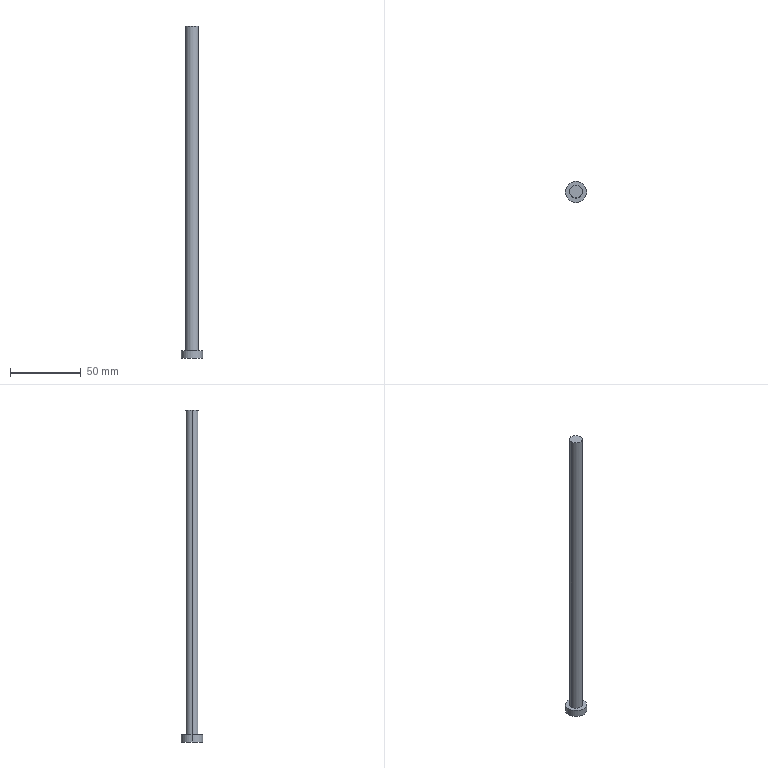Part | Creo | 1 solid | 7 faces | box 15 x 15 x 235 mm | volume 15516 mm3 | cylinder 4 | plane 3 | commonest cylinder face diameters 9 x2 15 x2
STEP:
#1=CARTESIAN_POINT('',(55.647,173.569,-230.5));
#2=VERTEX_POINT('',#1);
#3=CARTESIAN_POINT('',(64.647,173.569,-230.5));
#4=VERTEX_POINT('',#3);
#5=CARTESIAN_POINT('',(60.147,173.569,-230.5));
#6=DIRECTION('',(0.,0.,-1.));
#7=DIRECTION('',(-1.,0.,0.));
#8=AXIS2_PLACEMENT_3D('',#5,#6,#7);
#9=CIRCLE('',#8,4.5);
#10=EDGE_CURVE('',#2,#4,#9,.T.);
#11=ORIENTED_EDGE('',*,*,#10,.T.);
#12=CARTESIAN_POINT('',(64.647,173.569,-0.5));
#13=VERTEX_POINT('',#12);
#14=CARTESIAN_POINT('',(64.647,173.569,-230.5));
#15=DIRECTION('',(0.,0.,1.));
#16=VECTOR('',#15,230.);
#17=LINE('',#14,#16);
#18=EDGE_CURVE('',#4,#13,#17,.T.);
#19=ORIENTED_EDGE('',*,*,#18,.T.);
#20=CARTESIAN_POINT('',(55.647,173.569,-0.5));
#21=VERTEX_POINT('',#20);
#22=CARTESIAN_POINT('',(60.147,173.569,-0.5));
#23=DIRECTION('',(0.,0.,1.));
#24=DIRECTION('',(1.,0.,0.));
#25=AXIS2_PLACEMENT_3D('',#22,#23,#24);
#26=CIRCLE('',#25,4.5);
#27=EDGE_CURVE('',#13,#21,#26,.T.);
#28=ORIENTED_EDGE('',*,*,#27,.T.);
#29=CARTESIAN_POINT('',(55.647,173.569,-230.5));
#30=DIRECTION('',(0.,0.,1.));
#31=VECTOR('',#30,230.);
#32=LINE('',#29,#31);
#33=EDGE_CURVE('',#2,#21,#32,.T.);
#34=ORIENTED_EDGE('',*,*,#33,.F.);
#35=EDGE_LOOP('',(#11,#19,#28,#34));
#36=FACE_OUTER_BOUND('',#35,.F.);
#37=CARTESIAN_POINT('',(60.147,173.569,-250.296));
#38=DIRECTION('',(0.,0.,1.));
#39=DIRECTION('',(1.,0.,0.));
#40=AXIS2_PLACEMENT_3D('',#37,#38,#39);
#41=CYLINDRICAL_SURFACE('',#40,4.5);
#42=ADVANCED_FACE('',(#36),#41,.T.);
#43=CARTESIAN_POINT('',(67.647,173.569,-230.5));
#44=VERTEX_POINT('',#43);
#45=CARTESIAN_POINT('',(52.647,173.569,-230.5));
#46=VERTEX_POINT('',#45);
#47=CARTESIAN_POINT('',(60.147,173.569,-230.5));
#48=DIRECTION('',(0.,0.,1.));
#49=DIRECTION('',(1.,0.,0.));
#50=AXIS2_PLACEMENT_3D('',#47,#48,#49);
#51=CIRCLE('',#50,7.5);
#52=EDGE_CURVE('',#44,#46,#51,.T.);
#53=ORIENTED_EDGE('',*,*,#52,.F.);
#54=CARTESIAN_POINT('',(60.147,173.569,-230.5));
#55=DIRECTION('',(0.,0.,1.));
#56=DIRECTION('',(-1.,0.,0.));
#57=AXIS2_PLACEMENT_3D('',#54,#55,#56);
#58=CIRCLE('',#57,7.5);
#59=EDGE_CURVE('',#46,#44,#58,.T.);
#60=ORIENTED_EDGE('',*,*,#59,.F.);
#61=EDGE_LOOP('',(#53,#60));
#62=FACE_OUTER_BOUND('',#61,.F.);
#63=CARTESIAN_POINT('',(60.147,173.569,-230.5));
#64=DIRECTION('',(0.,0.,-1.));
#65=DIRECTION('',(1.,0.,0.));
#66=AXIS2_PLACEMENT_3D('',#63,#64,#65);
#67=CIRCLE('',#66,4.5);
#68=EDGE_CURVE('',#4,#2,#67,.T.);
#69=ORIENTED_EDGE('',*,*,#68,.F.);
#70=ORIENTED_EDGE('',*,*,#10,.F.);
#71=EDGE_LOOP('',(#69,#70));
#72=FACE_BOUND('',#71,.F.);
#73=CARTESIAN_POINT('',(60.147,173.569,-230.5));
#74=DIRECTION('',(0.,0.,1.));
#75=DIRECTION('',(1.,0.,0.));
#76=AXIS2_PLACEMENT_3D('',#73,#74,#75);
#77=PLANE('',#76);
#78=ADVANCED_FACE('',(#62,#72),#77,.T.);
#79=CARTESIAN_POINT('',(52.647,173.569,-235.5));
#80=VERTEX_POINT('',#79);
#81=CARTESIAN_POINT('',(67.647,173.569,-235.5));
#82=VERTEX_POINT('',#81);
#83=CARTESIAN_POINT('',(60.147,173.569,-235.5));
#84=DIRECTION('',(0.,0.,-1.));
#85=DIRECTION('',(-1.,0.,0.));
#86=AXIS2_PLACEMENT_3D('',#83,#84,#85);
#87=CIRCLE('',#86,7.5);
#88=EDGE_CURVE('',#80,#82,#87,.T.);
#89=ORIENTED_EDGE('',*,*,#88,.T.);
#90=CARTESIAN_POINT('',(67.647,173.569,-235.5));
#91=DIRECTION('',(0.,0.,1.));
#92=VECTOR('',#91,5.);
#93=LINE('',#90,#92);
#94=EDGE_CURVE('',#82,#44,#93,.T.);
#95=ORIENTED_EDGE('',*,*,#94,.T.);
#96=ORIENTED_EDGE('',*,*,#52,.T.);
#97=CARTESIAN_POINT('',(52.647,173.569,-235.5));
#98=DIRECTION('',(0.,0.,1.));
#99=VECTOR('',#98,5.);
#100=LINE('',#97,#99);
#101=EDGE_CURVE('',#80,#46,#100,.T.);
#102=ORIENTED_EDGE('',*,*,#101,.F.);
#103=EDGE_LOOP('',(#89,#95,#96,#102));
#104=FACE_OUTER_BOUND('',#103,.F.);
#105=CARTESIAN_POINT('',(60.147,173.569,-241.77));
#106=DIRECTION('',(0.,0.,1.));
#107=DIRECTION('',(1.,0.,0.));
#108=AXIS2_PLACEMENT_3D('',#105,#106,#107);
#109=CYLINDRICAL_SURFACE('',#108,7.5);
#110=ADVANCED_FACE('',(#104),#109,.T.);
#111=CARTESIAN_POINT('',(60.147,173.569,-235.5));
#112=DIRECTION('',(0.,0.,-1.));
#113=DIRECTION('',(1.,0.,0.));
#114=AXIS2_PLACEMENT_3D('',#111,#112,#113);
#115=CIRCLE('',#114,7.5);
#116=EDGE_CURVE('',#82,#80,#115,.T.);
#117=ORIENTED_EDGE('',*,*,#116,.F.);
#118=ORIENTED_EDGE('',*,*,#88,.F.);
#119=EDGE_LOOP('',(#117,#118));
#120=FACE_OUTER_BOUND('',#119,.F.);
#121=CARTESIAN_POINT('',(60.147,173.569,-235.5));
#122=DIRECTION('',(0.,0.,1.));
#123=DIRECTION('',(1.,0.,0.));
#124=AXIS2_PLACEMENT_3D('',#121,#122,#123);
#125=PLANE('',#124);
#126=ADVANCED_FACE('',(#120),#125,.F.);
#127=ORIENTED_EDGE('',*,*,#116,.T.);
#128=ORIENTED_EDGE('',*,*,#101,.T.);
#129=ORIENTED_EDGE('',*,*,#59,.T.);
#130=ORIENTED_EDGE('',*,*,#94,.F.);
#131=EDGE_LOOP('',(#127,#128,#129,#130));
#132=FACE_OUTER_BOUND('',#131,.F.);
#133=CARTESIAN_POINT('',(60.147,173.569,-241.77));
#134=DIRECTION('',(0.,0.,1.));
#135=DIRECTION('',(1.,0.,0.));
#136=AXIS2_PLACEMENT_3D('',#133,#134,#135);
#137=CYLINDRICAL_SURFACE('',#136,7.5);
#138=ADVANCED_FACE('',(#132),#137,.T.);
#139=ORIENTED_EDGE('',*,*,#68,.T.);
#140=ORIENTED_EDGE('',*,*,#33,.T.);
#141=CARTESIAN_POINT('',(60.147,173.569,-0.5));
#142=DIRECTION('',(0.,0.,1.));
#143=DIRECTION('',(-1.,0.,0.));
#144=AXIS2_PLACEMENT_3D('',#141,#142,#143);
#145=CIRCLE('',#144,4.5);
#146=EDGE_CURVE('',#21,#13,#145,.T.);
#147=ORIENTED_EDGE('',*,*,#146,.T.);
#148=ORIENTED_EDGE('',*,*,#18,.F.);
#149=EDGE_LOOP('',(#139,#140,#147,#148));
#150=FACE_OUTER_BOUND('',#149,.F.);
#151=CARTESIAN_POINT('',(60.147,173.569,-250.296));
#152=DIRECTION('',(0.,0.,1.));
#153=DIRECTION('',(1.,0.,0.));
#154=AXIS2_PLACEMENT_3D('',#151,#152,#153);
#155=CYLINDRICAL_SURFACE('',#154,4.5);
#156=ADVANCED_FACE('',(#150),#155,.T.);
#157=ORIENTED_EDGE('',*,*,#27,.F.);
#158=ORIENTED_EDGE('',*,*,#146,.F.);
#159=EDGE_LOOP('',(#157,#158));
#160=FACE_OUTER_BOUND('',#159,.F.);
#161=CARTESIAN_POINT('',(64.647,173.569,-0.5));
#162=DIRECTION('',(0.,0.,-1.));
#163=DIRECTION('',(-1.,0.,0.));
#164=AXIS2_PLACEMENT_3D('',#161,#162,#163);
#165=PLANE('',#164);
#166=ADVANCED_FACE('',(#160),#165,.F.);
#167=CLOSED_SHELL('',(#42,#78,#110,#126,#138,#156,#166));
#168=MANIFOLD_SOLID_BREP('',#167);
#169=(LENGTH_UNIT()NAMED_UNIT(*)SI_UNIT(.MILLI.,.METRE.));
#170=UNCERTAINTY_MEASURE_WITH_UNIT(LENGTH_MEASURE(0.02359),#169,'','');
#171=(NAMED_UNIT(*)PLANE_ANGLE_UNIT()SI_UNIT($,.RADIAN.));
#172=PLANE_ANGLE_MEASURE_WITH_UNIT(PLANE_ANGLE_MEASURE(0.01745),#171);
#173=(CONVERSION_BASED_UNIT('DEGREE',#172)NAMED_UNIT(*)PLANE_ANGLE_UNIT());
#174=(NAMED_UNIT(*)SI_UNIT($,.STERADIAN.)SOLID_ANGLE_UNIT());
#175=(GEOMETRIC_REPRESENTATION_CONTEXT(3)GLOBAL_UNCERTAINTY_ASSIGNED_CONTEXT((#170))GLOBAL_UNIT_ASSIGNED_CONTEXT((#169,#173,#174))REPRESENTATION_CONTEXT('',''));
#176=ADVANCED_BREP_SHAPE_REPRESENTATION('',(#168),#175);